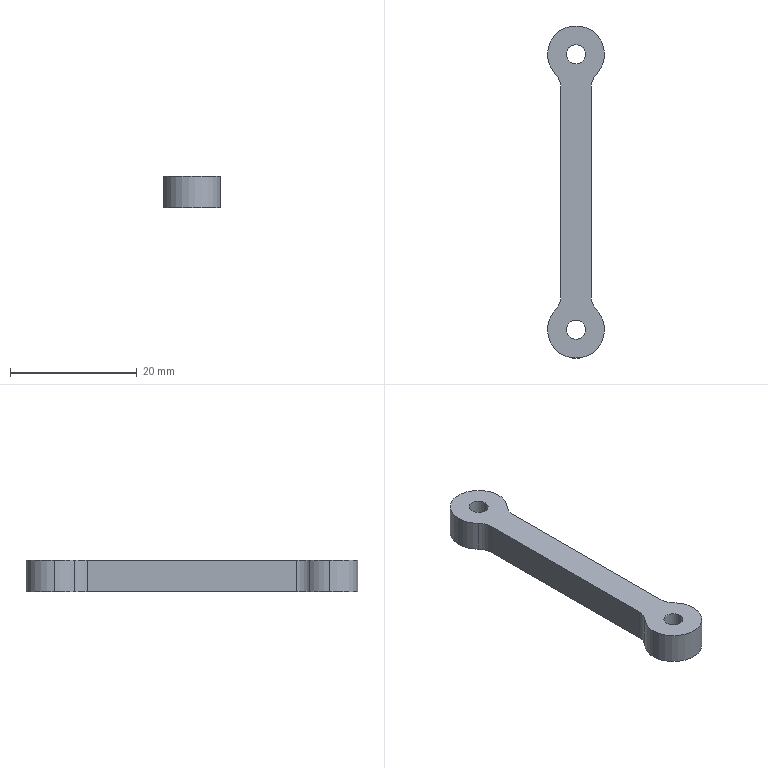Part | SolidWorks | features BaseBody 1 | 1 solid | 18 faces | box 9 x 52.5 x 5 mm | volume 1409 mm3 | cylinder 14 | plane 4 | commonest cylinder face diameters 9 x6 3 x4 6 x4
STEP:
#1=CARTESIAN_POINT('',(1.5,43.5,5.));
#2=VERTEX_POINT('',#1);
#3=CARTESIAN_POINT('',(1.5,43.5,0.));
#4=VERTEX_POINT('',#3);
#5=CARTESIAN_POINT('',(1.5,43.5,5.));
#6=DIRECTION('',(0.,0.,-1.));
#7=VECTOR('',#6,1000.);
#8=LINE('',#5,#7);
#9=EDGE_CURVE('',#2,#4,#8,.T.);
#10=ORIENTED_EDGE('',*,*,#9,.F.);
#11=CARTESIAN_POINT('',(-1.5,43.5,5.));
#12=VERTEX_POINT('',#11);
#13=CARTESIAN_POINT('',(0.,43.5,5.));
#14=DIRECTION('',(0.,0.,1.));
#15=DIRECTION('',(1.,0.,0.));
#16=AXIS2_PLACEMENT_3D('',#13,#14,#15);
#17=CIRCLE('',#16,1.5);
#18=EDGE_CURVE('',#2,#12,#17,.T.);
#19=ORIENTED_EDGE('',*,*,#18,.T.);
#20=CARTESIAN_POINT('',(-1.5,43.5,0.));
#21=VERTEX_POINT('',#20);
#22=CARTESIAN_POINT('',(-1.5,43.5,5.));
#23=DIRECTION('',(0.,0.,-1.));
#24=VECTOR('',#23,1000.);
#25=LINE('',#22,#24);
#26=EDGE_CURVE('',#12,#21,#25,.T.);
#27=ORIENTED_EDGE('',*,*,#26,.T.);
#28=CARTESIAN_POINT('',(0.,43.5,0.));
#29=DIRECTION('',(0.,0.,1.));
#30=DIRECTION('',(1.,0.,0.));
#31=AXIS2_PLACEMENT_3D('',#28,#29,#30);
#32=CIRCLE('',#31,1.5);
#33=EDGE_CURVE('',#4,#21,#32,.T.);
#34=ORIENTED_EDGE('',*,*,#33,.F.);
#35=EDGE_LOOP('',(#10,#19,#27,#34));
#36=FACE_OUTER_BOUND('',#35,.T.);
#37=CARTESIAN_POINT('',(0.,43.5,5.));
#38=DIRECTION('',(0.,0.,-1.));
#39=DIRECTION('',(-1.,0.,0.));
#40=AXIS2_PLACEMENT_3D('',#37,#38,#39);
#41=CYLINDRICAL_SURFACE('',#40,1.5);
#42=ADVANCED_FACE('',(#36),#41,.F.);
#43=CARTESIAN_POINT('',(1.5,0.,5.));
#44=VERTEX_POINT('',#43);
#45=CARTESIAN_POINT('',(1.5,0.,0.));
#46=VERTEX_POINT('',#45);
#47=CARTESIAN_POINT('',(1.5,0.,5.));
#48=DIRECTION('',(0.,0.,-1.));
#49=VECTOR('',#48,1000.);
#50=LINE('',#47,#49);
#51=EDGE_CURVE('',#44,#46,#50,.T.);
#52=ORIENTED_EDGE('',*,*,#51,.F.);
#53=CARTESIAN_POINT('',(-1.5,0.,5.));
#54=VERTEX_POINT('',#53);
#55=CARTESIAN_POINT('',(0.,0.,5.));
#56=DIRECTION('',(0.,0.,1.));
#57=DIRECTION('',(1.,0.,0.));
#58=AXIS2_PLACEMENT_3D('',#55,#56,#57);
#59=CIRCLE('',#58,1.5);
#60=EDGE_CURVE('',#44,#54,#59,.T.);
#61=ORIENTED_EDGE('',*,*,#60,.T.);
#62=CARTESIAN_POINT('',(-1.5,0.,0.));
#63=VERTEX_POINT('',#62);
#64=CARTESIAN_POINT('',(-1.5,0.,5.));
#65=DIRECTION('',(0.,0.,-1.));
#66=VECTOR('',#65,1000.);
#67=LINE('',#64,#66);
#68=EDGE_CURVE('',#54,#63,#67,.T.);
#69=ORIENTED_EDGE('',*,*,#68,.T.);
#70=CARTESIAN_POINT('',(0.,0.,0.));
#71=DIRECTION('',(0.,0.,1.));
#72=DIRECTION('',(1.,0.,0.));
#73=AXIS2_PLACEMENT_3D('',#70,#71,#72);
#74=CIRCLE('',#73,1.5);
#75=EDGE_CURVE('',#46,#63,#74,.T.);
#76=ORIENTED_EDGE('',*,*,#75,.F.);
#77=EDGE_LOOP('',(#52,#61,#69,#76));
#78=FACE_OUTER_BOUND('',#77,.T.);
#79=CARTESIAN_POINT('',(0.,0.,5.));
#80=DIRECTION('',(0.,0.,-1.));
#81=DIRECTION('',(-1.,0.,0.));
#82=AXIS2_PLACEMENT_3D('',#79,#80,#81);
#83=CYLINDRICAL_SURFACE('',#82,1.5);
#84=ADVANCED_FACE('',(#78),#83,.F.);
#85=CARTESIAN_POINT('',(-4.5,0.,5.));
#86=VERTEX_POINT('',#85);
#87=CARTESIAN_POINT('',(-4.5,0.,0.));
#88=VERTEX_POINT('',#87);
#89=CARTESIAN_POINT('',(-4.5,0.,5.));
#90=DIRECTION('',(0.,0.,-1.));
#91=VECTOR('',#90,1000.);
#92=LINE('',#89,#91);
#93=EDGE_CURVE('',#86,#88,#92,.T.);
#94=ORIENTED_EDGE('',*,*,#93,.F.);
#95=CARTESIAN_POINT('',(-3.24,3.123,5.));
#96=VERTEX_POINT('',#95);
#97=CARTESIAN_POINT('',(0.,0.,5.));
#98=DIRECTION('',(0.,0.,1.));
#99=DIRECTION('',(1.,0.,0.));
#100=AXIS2_PLACEMENT_3D('',#97,#98,#99);
#101=CIRCLE('',#100,4.5);
#102=EDGE_CURVE('',#96,#86,#101,.T.);
#103=ORIENTED_EDGE('',*,*,#102,.F.);
#104=CARTESIAN_POINT('',(-3.24,3.123,0.));
#105=VERTEX_POINT('',#104);
#106=CARTESIAN_POINT('',(-3.24,3.123,5.));
#107=DIRECTION('',(0.,0.,-1.));
#108=VECTOR('',#107,1000.);
#109=LINE('',#106,#108);
#110=EDGE_CURVE('',#96,#105,#109,.T.);
#111=ORIENTED_EDGE('',*,*,#110,.T.);
#112=CARTESIAN_POINT('',(0.,0.,0.));
#113=DIRECTION('',(0.,0.,1.));
#114=DIRECTION('',(1.,0.,0.));
#115=AXIS2_PLACEMENT_3D('',#112,#113,#114);
#116=CIRCLE('',#115,4.5);
#117=EDGE_CURVE('',#105,#88,#116,.T.);
#118=ORIENTED_EDGE('',*,*,#117,.T.);
#119=EDGE_LOOP('',(#94,#103,#111,#118));
#120=FACE_OUTER_BOUND('',#119,.T.);
#121=CARTESIAN_POINT('',(0.,0.,5.));
#122=DIRECTION('',(0.,0.,-1.));
#123=DIRECTION('',(-1.,0.,0.));
#124=AXIS2_PLACEMENT_3D('',#121,#122,#123);
#125=CYLINDRICAL_SURFACE('',#124,4.5);
#126=ADVANCED_FACE('',(#120),#125,.T.);
#127=CARTESIAN_POINT('',(-2.4,5.205,0.));
#128=VERTEX_POINT('',#127);
#129=CARTESIAN_POINT('',(-5.4,5.205,0.));
#130=DIRECTION('',(0.,0.,-1.));
#131=DIRECTION('',(1.,0.,0.));
#132=AXIS2_PLACEMENT_3D('',#129,#130,#131);
#133=CIRCLE('',#132,3.);
#134=EDGE_CURVE('',#128,#105,#133,.T.);
#135=ORIENTED_EDGE('',*,*,#134,.T.);
#136=ORIENTED_EDGE('',*,*,#110,.F.);
#137=CARTESIAN_POINT('',(-2.4,5.205,5.));
#138=VERTEX_POINT('',#137);
#139=CARTESIAN_POINT('',(-5.4,5.205,5.));
#140=DIRECTION('',(0.,0.,-1.));
#141=DIRECTION('',(1.,0.,0.));
#142=AXIS2_PLACEMENT_3D('',#139,#140,#141);
#143=CIRCLE('',#142,3.);
#144=EDGE_CURVE('',#138,#96,#143,.T.);
#145=ORIENTED_EDGE('',*,*,#144,.F.);
#146=CARTESIAN_POINT('',(-2.4,5.205,5.));
#147=DIRECTION('',(0.,0.,-1.));
#148=VECTOR('',#147,1000.);
#149=LINE('',#146,#148);
#150=EDGE_CURVE('',#138,#128,#149,.T.);
#151=ORIENTED_EDGE('',*,*,#150,.T.);
#152=EDGE_LOOP('',(#135,#136,#145,#151));
#153=FACE_OUTER_BOUND('',#152,.T.);
#154=CARTESIAN_POINT('',(-5.4,5.205,5.));
#155=DIRECTION('',(0.,0.,-1.));
#156=DIRECTION('',(-1.,0.,0.));
#157=AXIS2_PLACEMENT_3D('',#154,#155,#156);
#158=CYLINDRICAL_SURFACE('',#157,3.);
#159=ADVANCED_FACE('',(#153),#158,.F.);
#160=CARTESIAN_POINT('',(-2.4,38.295,0.));
#161=VERTEX_POINT('',#160);
#162=CARTESIAN_POINT('',(-2.4,38.295,0.));
#163=DIRECTION('',(0.,-1.,0.));
#164=VECTOR('',#163,1000.);
#165=LINE('',#162,#164);
#166=EDGE_CURVE('',#161,#128,#165,.T.);
#167=ORIENTED_EDGE('',*,*,#166,.T.);
#168=ORIENTED_EDGE('',*,*,#150,.F.);
#169=CARTESIAN_POINT('',(-2.4,38.295,5.));
#170=VERTEX_POINT('',#169);
#171=CARTESIAN_POINT('',(-2.4,38.295,5.));
#172=DIRECTION('',(0.,-1.,0.));
#173=VECTOR('',#172,1000.);
#174=LINE('',#171,#173);
#175=EDGE_CURVE('',#170,#138,#174,.T.);
#176=ORIENTED_EDGE('',*,*,#175,.F.);
#177=CARTESIAN_POINT('',(-2.4,38.295,5.));
#178=DIRECTION('',(0.,0.,-1.));
#179=VECTOR('',#178,1000.);
#180=LINE('',#177,#179);
#181=EDGE_CURVE('',#170,#161,#180,.T.);
#182=ORIENTED_EDGE('',*,*,#181,.T.);
#183=EDGE_LOOP('',(#167,#168,#176,#182));
#184=FACE_OUTER_BOUND('',#183,.T.);
#185=CARTESIAN_POINT('',(-2.4,38.295,5.));
#186=DIRECTION('',(1.,0.,0.));
#187=DIRECTION('',(0.,1.,0.));
#188=AXIS2_PLACEMENT_3D('',#185,#186,#187);
#189=PLANE('',#188);
#190=ADVANCED_FACE('',(#184),#189,.F.);
#191=CARTESIAN_POINT('',(-3.24,40.377,0.));
#192=VERTEX_POINT('',#191);
#193=CARTESIAN_POINT('',(-5.4,38.295,0.));
#194=DIRECTION('',(0.,0.,-1.));
#195=DIRECTION('',(1.,0.,0.));
#196=AXIS2_PLACEMENT_3D('',#193,#194,#195);
#197=CIRCLE('',#196,3.);
#198=EDGE_CURVE('',#192,#161,#197,.T.);
#199=ORIENTED_EDGE('',*,*,#198,.T.);
#200=ORIENTED_EDGE('',*,*,#181,.F.);
#201=CARTESIAN_POINT('',(-3.24,40.377,5.));
#202=VERTEX_POINT('',#201);
#203=CARTESIAN_POINT('',(-5.4,38.295,5.));
#204=DIRECTION('',(0.,0.,-1.));
#205=DIRECTION('',(1.,0.,0.));
#206=AXIS2_PLACEMENT_3D('',#203,#204,#205);
#207=CIRCLE('',#206,3.);
#208=EDGE_CURVE('',#202,#170,#207,.T.);
#209=ORIENTED_EDGE('',*,*,#208,.F.);
#210=CARTESIAN_POINT('',(-3.24,40.377,5.));
#211=DIRECTION('',(0.,0.,-1.));
#212=VECTOR('',#211,1000.);
#213=LINE('',#210,#212);
#214=EDGE_CURVE('',#202,#192,#213,.T.);
#215=ORIENTED_EDGE('',*,*,#214,.T.);
#216=EDGE_LOOP('',(#199,#200,#209,#215));
#217=FACE_OUTER_BOUND('',#216,.T.);
#218=CARTESIAN_POINT('',(-5.4,38.295,5.));
#219=DIRECTION('',(0.,0.,-1.));
#220=DIRECTION('',(-1.,0.,0.));
#221=AXIS2_PLACEMENT_3D('',#218,#219,#220);
#222=CYLINDRICAL_SURFACE('',#221,3.);
#223=ADVANCED_FACE('',(#217),#222,.F.);
#224=CARTESIAN_POINT('',(4.5,43.5,5.));
#225=VERTEX_POINT('',#224);
#226=CARTESIAN_POINT('',(4.5,43.5,0.));
#227=VERTEX_POINT('',#226);
#228=CARTESIAN_POINT('',(4.5,43.5,5.));
#229=DIRECTION('',(0.,0.,-1.));
#230=VECTOR('',#229,1000.);
#231=LINE('',#228,#230);
#232=EDGE_CURVE('',#225,#227,#231,.T.);
#233=ORIENTED_EDGE('',*,*,#232,.F.);
#234=CARTESIAN_POINT('',(3.24,40.377,5.));
#235=VERTEX_POINT('',#234);
#236=CARTESIAN_POINT('',(0.,43.5,5.));
#237=DIRECTION('',(0.,0.,1.));
#238=DIRECTION('',(1.,0.,0.));
#239=AXIS2_PLACEMENT_3D('',#236,#237,#238);
#240=CIRCLE('',#239,4.5);
#241=EDGE_CURVE('',#235,#225,#240,.T.);
#242=ORIENTED_EDGE('',*,*,#241,.F.);
#243=CARTESIAN_POINT('',(3.24,40.377,0.));
#244=VERTEX_POINT('',#243);
#245=CARTESIAN_POINT('',(3.24,40.377,5.));
#246=DIRECTION('',(0.,0.,-1.));
#247=VECTOR('',#246,1000.);
#248=LINE('',#245,#247);
#249=EDGE_CURVE('',#235,#244,#248,.T.);
#250=ORIENTED_EDGE('',*,*,#249,.T.);
#251=CARTESIAN_POINT('',(0.,43.5,0.));
#252=DIRECTION('',(0.,0.,1.));
#253=DIRECTION('',(1.,0.,0.));
#254=AXIS2_PLACEMENT_3D('',#251,#252,#253);
#255=CIRCLE('',#254,4.5);
#256=EDGE_CURVE('',#244,#227,#255,.T.);
#257=ORIENTED_EDGE('',*,*,#256,.T.);
#258=EDGE_LOOP('',(#233,#242,#250,#257));
#259=FACE_OUTER_BOUND('',#258,.T.);
#260=CARTESIAN_POINT('',(0.,43.5,5.));
#261=DIRECTION('',(0.,0.,-1.));
#262=DIRECTION('',(-1.,0.,0.));
#263=AXIS2_PLACEMENT_3D('',#260,#261,#262);
#264=CYLINDRICAL_SURFACE('',#263,4.5);
#265=ADVANCED_FACE('',(#259),#264,.T.);
#266=CARTESIAN_POINT('',(2.4,38.295,0.));
#267=VERTEX_POINT('',#266);
#268=CARTESIAN_POINT('',(5.4,38.295,0.));
#269=DIRECTION('',(0.,0.,-1.));
#270=DIRECTION('',(1.,0.,0.));
#271=AXIS2_PLACEMENT_3D('',#268,#269,#270);
#272=CIRCLE('',#271,3.);
#273=EDGE_CURVE('',#267,#244,#272,.T.);
#274=ORIENTED_EDGE('',*,*,#273,.T.);
#275=ORIENTED_EDGE('',*,*,#249,.F.);
#276=CARTESIAN_POINT('',(2.4,38.295,5.));
#277=VERTEX_POINT('',#276);
#278=CARTESIAN_POINT('',(5.4,38.295,5.));
#279=DIRECTION('',(0.,0.,-1.));
#280=DIRECTION('',(1.,0.,0.));
#281=AXIS2_PLACEMENT_3D('',#278,#279,#280);
#282=CIRCLE('',#281,3.);
#283=EDGE_CURVE('',#277,#235,#282,.T.);
#284=ORIENTED_EDGE('',*,*,#283,.F.);
#285=CARTESIAN_POINT('',(2.4,38.295,5.));
#286=DIRECTION('',(0.,0.,-1.));
#287=VECTOR('',#286,1000.);
#288=LINE('',#285,#287);
#289=EDGE_CURVE('',#277,#267,#288,.T.);
#290=ORIENTED_EDGE('',*,*,#289,.T.);
#291=EDGE_LOOP('',(#274,#275,#284,#290));
#292=FACE_OUTER_BOUND('',#291,.T.);
#293=CARTESIAN_POINT('',(5.4,38.295,5.));
#294=DIRECTION('',(0.,0.,-1.));
#295=DIRECTION('',(-1.,0.,0.));
#296=AXIS2_PLACEMENT_3D('',#293,#294,#295);
#297=CYLINDRICAL_SURFACE('',#296,3.);
#298=ADVANCED_FACE('',(#292),#297,.F.);
#299=CARTESIAN_POINT('',(2.4,5.205,0.));
#300=VERTEX_POINT('',#299);
#301=CARTESIAN_POINT('',(2.4,38.295,0.));
#302=DIRECTION('',(0.,1.,0.));
#303=VECTOR('',#302,1000.);
#304=LINE('',#301,#303);
#305=EDGE_CURVE('',#300,#267,#304,.T.);
#306=ORIENTED_EDGE('',*,*,#305,.T.);
#307=ORIENTED_EDGE('',*,*,#289,.F.);
#308=CARTESIAN_POINT('',(2.4,5.205,5.));
#309=VERTEX_POINT('',#308);
#310=CARTESIAN_POINT('',(2.4,38.295,5.));
#311=DIRECTION('',(0.,1.,0.));
#312=VECTOR('',#311,1000.);
#313=LINE('',#310,#312);
#314=EDGE_CURVE('',#309,#277,#313,.T.);
#315=ORIENTED_EDGE('',*,*,#314,.F.);
#316=CARTESIAN_POINT('',(2.4,5.205,5.));
#317=DIRECTION('',(0.,0.,-1.));
#318=VECTOR('',#317,1000.);
#319=LINE('',#316,#318);
#320=EDGE_CURVE('',#309,#300,#319,.T.);
#321=ORIENTED_EDGE('',*,*,#320,.T.);
#322=EDGE_LOOP('',(#306,#307,#315,#321));
#323=FACE_OUTER_BOUND('',#322,.T.);
#324=CARTESIAN_POINT('',(2.4,38.295,5.));
#325=DIRECTION('',(-1.,0.,0.));
#326=DIRECTION('',(0.,1.,0.));
#327=AXIS2_PLACEMENT_3D('',#324,#325,#326);
#328=PLANE('',#327);
#329=ADVANCED_FACE('',(#323),#328,.F.);
#330=CARTESIAN_POINT('',(3.24,3.123,0.));
#331=VERTEX_POINT('',#330);
#332=CARTESIAN_POINT('',(5.4,5.205,0.));
#333=DIRECTION('',(0.,0.,-1.));
#334=DIRECTION('',(-1.,0.,0.));
#335=AXIS2_PLACEMENT_3D('',#332,#333,#334);
#336=CIRCLE('',#335,3.);
#337=EDGE_CURVE('',#331,#300,#336,.T.);
#338=ORIENTED_EDGE('',*,*,#337,.T.);
#339=ORIENTED_EDGE('',*,*,#320,.F.);
#340=CARTESIAN_POINT('',(3.24,3.123,5.));
#341=VERTEX_POINT('',#340);
#342=CARTESIAN_POINT('',(5.4,5.205,5.));
#343=DIRECTION('',(0.,0.,-1.));
#344=DIRECTION('',(-1.,0.,0.));
#345=AXIS2_PLACEMENT_3D('',#342,#343,#344);
#346=CIRCLE('',#345,3.);
#347=EDGE_CURVE('',#341,#309,#346,.T.);
#348=ORIENTED_EDGE('',*,*,#347,.F.);
#349=CARTESIAN_POINT('',(3.24,3.123,5.));
#350=DIRECTION('',(0.,0.,-1.));
#351=VECTOR('',#350,1000.);
#352=LINE('',#349,#351);
#353=EDGE_CURVE('',#341,#331,#352,.T.);
#354=ORIENTED_EDGE('',*,*,#353,.T.);
#355=EDGE_LOOP('',(#338,#339,#348,#354));
#356=FACE_OUTER_BOUND('',#355,.T.);
#357=CARTESIAN_POINT('',(5.4,5.205,5.));
#358=DIRECTION('',(0.,0.,-1.));
#359=DIRECTION('',(-1.,0.,0.));
#360=AXIS2_PLACEMENT_3D('',#357,#358,#359);
#361=CYLINDRICAL_SURFACE('',#360,3.);
#362=ADVANCED_FACE('',(#356),#361,.F.);
#363=CARTESIAN_POINT('',(0.,43.5,0.));
#364=DIRECTION('',(0.,0.,1.));
#365=DIRECTION('',(1.,0.,0.));
#366=AXIS2_PLACEMENT_3D('',#363,#364,#365);
#367=CIRCLE('',#366,1.5);
#368=EDGE_CURVE('',#21,#4,#367,.T.);
#369=ORIENTED_EDGE('',*,*,#368,.T.);
#370=ORIENTED_EDGE('',*,*,#33,.T.);
#371=EDGE_LOOP('',(#369,#370));
#372=FACE_BOUND('',#371,.T.);
#373=CARTESIAN_POINT('',(0.,0.,0.));
#374=DIRECTION('',(0.,0.,1.));
#375=DIRECTION('',(1.,0.,0.));
#376=AXIS2_PLACEMENT_3D('',#373,#374,#375);
#377=CIRCLE('',#376,1.5);
#378=EDGE_CURVE('',#63,#46,#377,.T.);
#379=ORIENTED_EDGE('',*,*,#378,.T.);
#380=ORIENTED_EDGE('',*,*,#75,.T.);
#381=EDGE_LOOP('',(#379,#380));
#382=FACE_BOUND('',#381,.T.);
#383=ORIENTED_EDGE('',*,*,#337,.F.);
#384=CARTESIAN_POINT('',(4.5,0.,0.));
#385=VERTEX_POINT('',#384);
#386=CARTESIAN_POINT('',(0.,0.,0.));
#387=DIRECTION('',(0.,0.,1.));
#388=DIRECTION('',(1.,0.,0.));
#389=AXIS2_PLACEMENT_3D('',#386,#387,#388);
#390=CIRCLE('',#389,4.5);
#391=EDGE_CURVE('',#385,#331,#390,.T.);
#392=ORIENTED_EDGE('',*,*,#391,.F.);
#393=CARTESIAN_POINT('',(0.,0.,0.));
#394=DIRECTION('',(0.,0.,1.));
#395=DIRECTION('',(1.,0.,0.));
#396=AXIS2_PLACEMENT_3D('',#393,#394,#395);
#397=CIRCLE('',#396,4.5);
#398=EDGE_CURVE('',#88,#385,#397,.T.);
#399=ORIENTED_EDGE('',*,*,#398,.F.);
#400=ORIENTED_EDGE('',*,*,#117,.F.);
#401=ORIENTED_EDGE('',*,*,#134,.F.);
#402=ORIENTED_EDGE('',*,*,#166,.F.);
#403=ORIENTED_EDGE('',*,*,#198,.F.);
#404=CARTESIAN_POINT('',(-4.5,43.5,0.));
#405=VERTEX_POINT('',#404);
#406=CARTESIAN_POINT('',(0.,43.5,0.));
#407=DIRECTION('',(0.,0.,1.));
#408=DIRECTION('',(1.,0.,0.));
#409=AXIS2_PLACEMENT_3D('',#406,#407,#408);
#410=CIRCLE('',#409,4.5);
#411=EDGE_CURVE('',#405,#192,#410,.T.);
#412=ORIENTED_EDGE('',*,*,#411,.F.);
#413=CARTESIAN_POINT('',(0.,43.5,0.));
#414=DIRECTION('',(0.,0.,1.));
#415=DIRECTION('',(1.,0.,0.));
#416=AXIS2_PLACEMENT_3D('',#413,#414,#415);
#417=CIRCLE('',#416,4.5);
#418=EDGE_CURVE('',#227,#405,#417,.T.);
#419=ORIENTED_EDGE('',*,*,#418,.F.);
#420=ORIENTED_EDGE('',*,*,#256,.F.);
#421=ORIENTED_EDGE('',*,*,#273,.F.);
#422=ORIENTED_EDGE('',*,*,#305,.F.);
#423=EDGE_LOOP('',(#383,#392,#399,#400,#401,#402,#403,#412,#419,#420,#421,#422));
#424=FACE_OUTER_BOUND('',#423,.T.);
#425=CARTESIAN_POINT('',(5.4,5.205,0.));
#426=DIRECTION('',(0.,0.,-1.));
#427=DIRECTION('',(0.,-1.,0.));
#428=AXIS2_PLACEMENT_3D('',#425,#426,#427);
#429=PLANE('',#428);
#430=ADVANCED_FACE('',(#372,#382,#424),#429,.T.);
#431=CARTESIAN_POINT('',(0.,43.5,5.));
#432=DIRECTION('',(0.,0.,1.));
#433=DIRECTION('',(1.,0.,0.));
#434=AXIS2_PLACEMENT_3D('',#431,#432,#433);
#435=CIRCLE('',#434,1.5);
#436=EDGE_CURVE('',#12,#2,#435,.T.);
#437=ORIENTED_EDGE('',*,*,#436,.F.);
#438=ORIENTED_EDGE('',*,*,#18,.F.);
#439=EDGE_LOOP('',(#437,#438));
#440=FACE_BOUND('',#439,.T.);
#441=CARTESIAN_POINT('',(0.,0.,5.));
#442=DIRECTION('',(0.,0.,1.));
#443=DIRECTION('',(1.,0.,0.));
#444=AXIS2_PLACEMENT_3D('',#441,#442,#443);
#445=CIRCLE('',#444,1.5);
#446=EDGE_CURVE('',#54,#44,#445,.T.);
#447=ORIENTED_EDGE('',*,*,#446,.F.);
#448=ORIENTED_EDGE('',*,*,#60,.F.);
#449=EDGE_LOOP('',(#447,#448));
#450=FACE_BOUND('',#449,.T.);
#451=ORIENTED_EDGE('',*,*,#347,.T.);
#452=ORIENTED_EDGE('',*,*,#314,.T.);
#453=ORIENTED_EDGE('',*,*,#283,.T.);
#454=ORIENTED_EDGE('',*,*,#241,.T.);
#455=CARTESIAN_POINT('',(-4.5,43.5,5.));
#456=VERTEX_POINT('',#455);
#457=CARTESIAN_POINT('',(0.,43.5,5.));
#458=DIRECTION('',(0.,0.,1.));
#459=DIRECTION('',(1.,0.,0.));
#460=AXIS2_PLACEMENT_3D('',#457,#458,#459);
#461=CIRCLE('',#460,4.5);
#462=EDGE_CURVE('',#225,#456,#461,.T.);
#463=ORIENTED_EDGE('',*,*,#462,.T.);
#464=CARTESIAN_POINT('',(0.,43.5,5.));
#465=DIRECTION('',(0.,0.,1.));
#466=DIRECTION('',(1.,0.,0.));
#467=AXIS2_PLACEMENT_3D('',#464,#465,#466);
#468=CIRCLE('',#467,4.5);
#469=EDGE_CURVE('',#456,#202,#468,.T.);
#470=ORIENTED_EDGE('',*,*,#469,.T.);
#471=ORIENTED_EDGE('',*,*,#208,.T.);
#472=ORIENTED_EDGE('',*,*,#175,.T.);
#473=ORIENTED_EDGE('',*,*,#144,.T.);
#474=ORIENTED_EDGE('',*,*,#102,.T.);
#475=CARTESIAN_POINT('',(4.5,0.,5.));
#476=VERTEX_POINT('',#475);
#477=CARTESIAN_POINT('',(0.,0.,5.));
#478=DIRECTION('',(0.,0.,1.));
#479=DIRECTION('',(1.,0.,0.));
#480=AXIS2_PLACEMENT_3D('',#477,#478,#479);
#481=CIRCLE('',#480,4.5);
#482=EDGE_CURVE('',#86,#476,#481,.T.);
#483=ORIENTED_EDGE('',*,*,#482,.T.);
#484=CARTESIAN_POINT('',(0.,0.,5.));
#485=DIRECTION('',(0.,0.,1.));
#486=DIRECTION('',(1.,0.,0.));
#487=AXIS2_PLACEMENT_3D('',#484,#485,#486);
#488=CIRCLE('',#487,4.5);
#489=EDGE_CURVE('',#476,#341,#488,.T.);
#490=ORIENTED_EDGE('',*,*,#489,.T.);
#491=EDGE_LOOP('',(#451,#452,#453,#454,#463,#470,#471,#472,#473,#474,#483,#490));
#492=FACE_OUTER_BOUND('',#491,.T.);
#493=CARTESIAN_POINT('',(5.4,5.205,5.));
#494=DIRECTION('',(0.,0.,-1.));
#495=DIRECTION('',(0.,-1.,0.));
#496=AXIS2_PLACEMENT_3D('',#493,#494,#495);
#497=PLANE('',#496);
#498=ADVANCED_FACE('',(#440,#450,#492),#497,.F.);
#499=ORIENTED_EDGE('',*,*,#469,.F.);
#500=CARTESIAN_POINT('',(-4.5,43.5,5.));
#501=DIRECTION('',(0.,0.,-1.));
#502=VECTOR('',#501,1000.);
#503=LINE('',#500,#502);
#504=EDGE_CURVE('',#456,#405,#503,.T.);
#505=ORIENTED_EDGE('',*,*,#504,.T.);
#506=ORIENTED_EDGE('',*,*,#411,.T.);
#507=ORIENTED_EDGE('',*,*,#214,.F.);
#508=EDGE_LOOP('',(#499,#505,#506,#507));
#509=FACE_OUTER_BOUND('',#508,.T.);
#510=CARTESIAN_POINT('',(0.,43.5,5.));
#511=DIRECTION('',(0.,0.,-1.));
#512=DIRECTION('',(-1.,0.,0.));
#513=AXIS2_PLACEMENT_3D('',#510,#511,#512);
#514=CYLINDRICAL_SURFACE('',#513,4.5);
#515=ADVANCED_FACE('',(#509),#514,.T.);
#516=ORIENTED_EDGE('',*,*,#462,.F.);
#517=ORIENTED_EDGE('',*,*,#232,.T.);
#518=ORIENTED_EDGE('',*,*,#418,.T.);
#519=ORIENTED_EDGE('',*,*,#504,.F.);
#520=EDGE_LOOP('',(#516,#517,#518,#519));
#521=FACE_OUTER_BOUND('',#520,.T.);
#522=CARTESIAN_POINT('',(0.,43.5,5.));
#523=DIRECTION('',(0.,0.,-1.));
#524=DIRECTION('',(-1.,0.,0.));
#525=AXIS2_PLACEMENT_3D('',#522,#523,#524);
#526=CYLINDRICAL_SURFACE('',#525,4.5);
#527=ADVANCED_FACE('',(#521),#526,.T.);
#528=CARTESIAN_POINT('',(4.5,0.,5.));
#529=DIRECTION('',(0.,0.,-1.));
#530=VECTOR('',#529,1000.);
#531=LINE('',#528,#530);
#532=EDGE_CURVE('',#476,#385,#531,.T.);
#533=ORIENTED_EDGE('',*,*,#532,.F.);
#534=ORIENTED_EDGE('',*,*,#482,.F.);
#535=ORIENTED_EDGE('',*,*,#93,.T.);
#536=ORIENTED_EDGE('',*,*,#398,.T.);
#537=EDGE_LOOP('',(#533,#534,#535,#536));
#538=FACE_OUTER_BOUND('',#537,.T.);
#539=CARTESIAN_POINT('',(0.,0.,5.));
#540=DIRECTION('',(0.,0.,-1.));
#541=DIRECTION('',(-1.,0.,0.));
#542=AXIS2_PLACEMENT_3D('',#539,#540,#541);
#543=CYLINDRICAL_SURFACE('',#542,4.5);
#544=ADVANCED_FACE('',(#538),#543,.T.);
#545=ORIENTED_EDGE('',*,*,#489,.F.);
#546=ORIENTED_EDGE('',*,*,#532,.T.);
#547=ORIENTED_EDGE('',*,*,#391,.T.);
#548=ORIENTED_EDGE('',*,*,#353,.F.);
#549=EDGE_LOOP('',(#545,#546,#547,#548));
#550=FACE_OUTER_BOUND('',#549,.T.);
#551=CARTESIAN_POINT('',(0.,0.,5.));
#552=DIRECTION('',(0.,0.,-1.));
#553=DIRECTION('',(-1.,0.,0.));
#554=AXIS2_PLACEMENT_3D('',#551,#552,#553);
#555=CYLINDRICAL_SURFACE('',#554,4.5);
#556=ADVANCED_FACE('',(#550),#555,.T.);
#557=ORIENTED_EDGE('',*,*,#446,.T.);
#558=ORIENTED_EDGE('',*,*,#51,.T.);
#559=ORIENTED_EDGE('',*,*,#378,.F.);
#560=ORIENTED_EDGE('',*,*,#68,.F.);
#561=EDGE_LOOP('',(#557,#558,#559,#560));
#562=FACE_OUTER_BOUND('',#561,.T.);
#563=CARTESIAN_POINT('',(0.,0.,5.));
#564=DIRECTION('',(0.,0.,-1.));
#565=DIRECTION('',(-1.,0.,0.));
#566=AXIS2_PLACEMENT_3D('',#563,#564,#565);
#567=CYLINDRICAL_SURFACE('',#566,1.5);
#568=ADVANCED_FACE('',(#562),#567,.F.);
#569=ORIENTED_EDGE('',*,*,#436,.T.);
#570=ORIENTED_EDGE('',*,*,#9,.T.);
#571=ORIENTED_EDGE('',*,*,#368,.F.);
#572=ORIENTED_EDGE('',*,*,#26,.F.);
#573=EDGE_LOOP('',(#569,#570,#571,#572));
#574=FACE_OUTER_BOUND('',#573,.T.);
#575=CARTESIAN_POINT('',(0.,43.5,5.));
#576=DIRECTION('',(0.,0.,-1.));
#577=DIRECTION('',(-1.,0.,0.));
#578=AXIS2_PLACEMENT_3D('',#575,#576,#577);
#579=CYLINDRICAL_SURFACE('',#578,1.5);
#580=ADVANCED_FACE('',(#574),#579,.F.);
#581=CLOSED_SHELL('',(#42,#84,#126,#159,#190,#223,#265,#298,#329,#362,#430,#498,#515,#527,#544,#556,#568,#580));
#582=MANIFOLD_SOLID_BREP('',#581);
#583=CARTESIAN_POINT('',(0.,0.,0.));
#584=DIRECTION('',(0.,0.,1.));
#585=DIRECTION('',(1.,0.,0.));
#586=AXIS2_PLACEMENT_3D('',#583,#584,#585);
#587=(LENGTH_UNIT()NAMED_UNIT(*)SI_UNIT(.MILLI.,.METRE.));
#588=UNCERTAINTY_MEASURE_WITH_UNIT(LENGTH_MEASURE(0.00001),#587,'','');
#589=(NAMED_UNIT(*)PLANE_ANGLE_UNIT()SI_UNIT($,.RADIAN.));
#590=(NAMED_UNIT(*)SI_UNIT($,.STERADIAN.)SOLID_ANGLE_UNIT());
#591=(GEOMETRIC_REPRESENTATION_CONTEXT(3)GLOBAL_UNCERTAINTY_ASSIGNED_CONTEXT((#588))GLOBAL_UNIT_ASSIGNED_CONTEXT((#587,#589,#590))REPRESENTATION_CONTEXT('',''));
#592=ADVANCED_BREP_SHAPE_REPRESENTATION('',(#582,#586),#591);